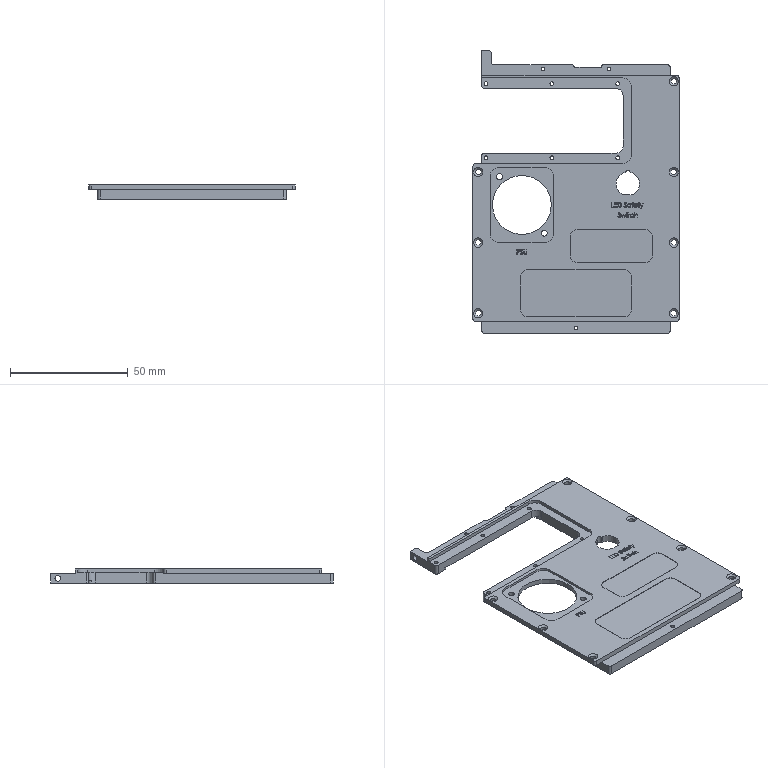NC program | NX | posted with a generic post | part box 87.5 x 120 x 6.001 mm
Lines 1 to 20 of 10039:
N10 G17 G21 G94 G90
(FLOOR_WALL , TOOL : D63面刀)
N12 T01 M6
N14 G53
N16 G17 G0 G90 X-101.5 Y24.25 B0. C0. S4500 M3
N18 G43 Z50. H1
N20 Z3.
N22 G94 G1 Z0. F700.
N24 X-91.5
N26 X91.5
N28 Y-14.8
N30 X-91.5
N32 X-101.5
N34 Z3.
N36 G0 Z50.
N38 M5